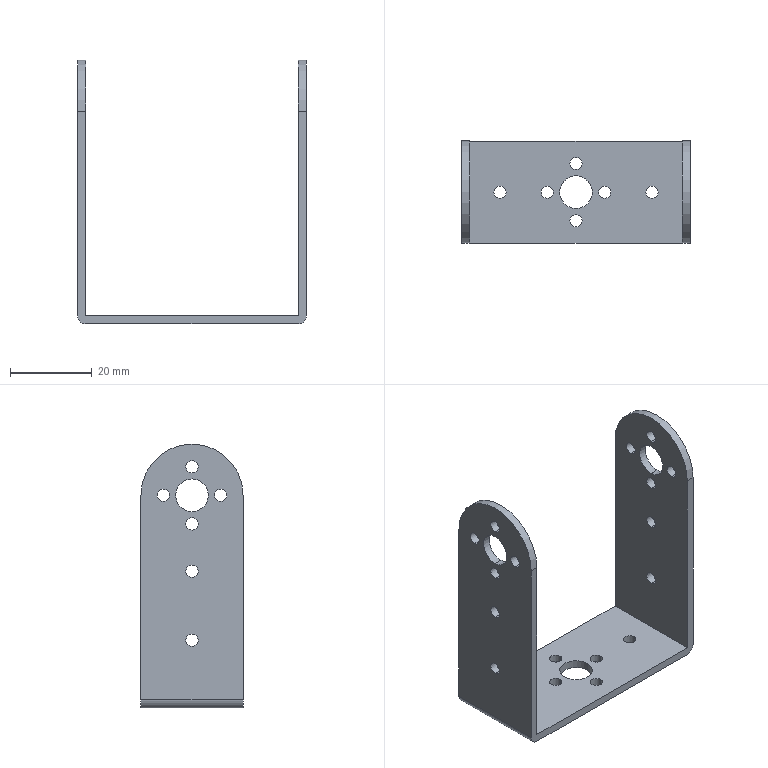Part | STEP file | U long bracket | 1 solid | 54 faces | box 56 x 25 x 64.5 mm | volume 8183 mm3 | cylinder 46 | plane 8 | commonest cylinder face diameters 3 x36 8 x6 4 x2 25 x2